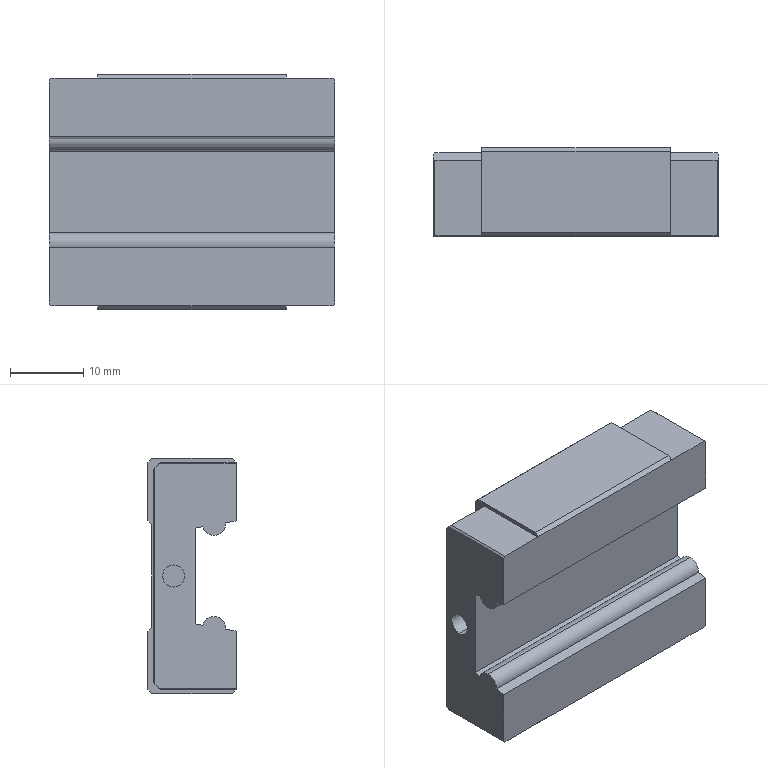Part | STEP file | RSR15M1V1Slider(2)^SRS15MUU-220LM-G10_Buffer motion shaft | 1 solid | 71 faces | box 38.9 x 12 x 32 mm | volume 11407 mm3 | plane 40 | cone 16 | cylinder 15 | commonest cylinder face diameters 2.459 x8 3 x4 3.18 x3